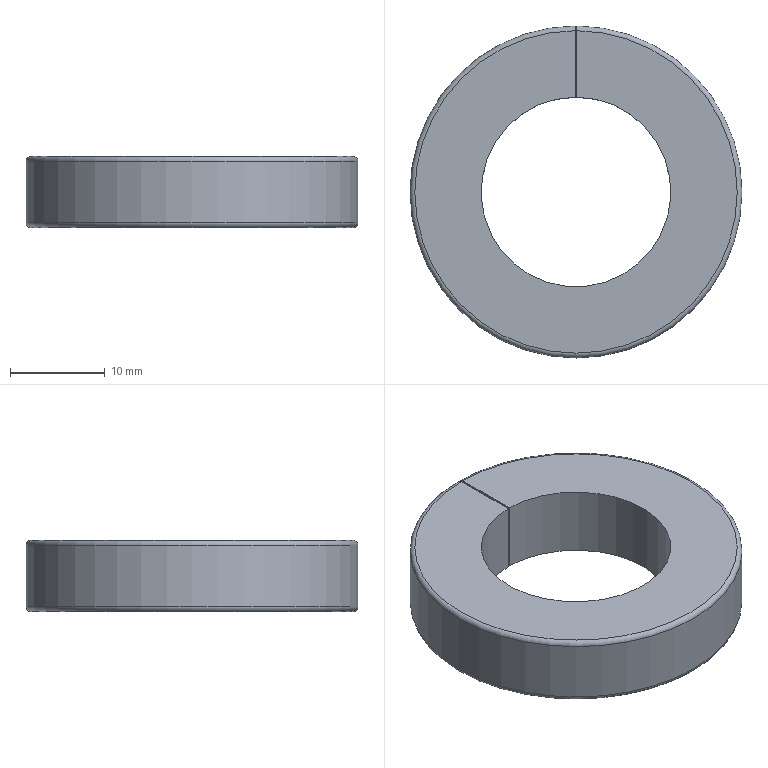Part | NX | features DATUM_CSYS 2, BLEND 1, EXTRUDE 1, SKETCH 1 | 1 solid | 8 faces | box 35 x 35 x 7.5 mm | volume 4837 mm3 | plane 4 | cylinder 2 | torus 2 | commonest cylinder face diameters 20 x1 35 x1
STEP:
#1=CARTESIAN_POINT('',(-0.1,9.999,0.));
#2=VERTEX_POINT('',#1);
#3=CARTESIAN_POINT('',(-0.1,17.,0.));
#4=VERTEX_POINT('',#3);
#5=CARTESIAN_POINT('',(-0.1,9.999,0.));
#6=DIRECTION('',(0.,1.,0.));
#7=VECTOR('',#6,1000.);
#8=LINE('',#5,#7);
#9=EDGE_CURVE('',#2,#4,#8,.T.);
#10=ORIENTED_EDGE('',*,*,#9,.T.);
#11=CARTESIAN_POINT('',(-0.1,17.5,0.5));
#12=VERTEX_POINT('',#11);
#13=CARTESIAN_POINT('',(-0.1,17.,0.));
#14=CARTESIAN_POINT('',(-0.1,17.264,0.));
#15=CARTESIAN_POINT('',(-0.1,17.5,0.2359));
#16=CARTESIAN_POINT('',(-0.1,17.5,0.5));
#17=B_SPLINE_CURVE_WITH_KNOTS('',3,(#13,#14,#15,#16),.UNSPECIFIED.,.F.,.F.,(4,4),(0.,0.0007811),.UNSPECIFIED.);
#18=EDGE_CURVE('',#4,#12,#17,.T.);
#19=ORIENTED_EDGE('',*,*,#18,.T.);
#20=CARTESIAN_POINT('',(-0.1,17.5,7.));
#21=VERTEX_POINT('',#20);
#22=CARTESIAN_POINT('',(-0.1,17.5,7.5));
#23=DIRECTION('',(0.,0.,-1.));
#24=VECTOR('',#23,1000.);
#25=LINE('',#22,#24);
#26=EDGE_CURVE('',#21,#12,#25,.T.);
#27=ORIENTED_EDGE('',*,*,#26,.F.);
#28=CARTESIAN_POINT('',(-0.1,17.,7.5));
#29=VERTEX_POINT('',#28);
#30=CARTESIAN_POINT('',(-0.1,17.5,7.));
#31=CARTESIAN_POINT('',(-0.1,17.5,7.264));
#32=CARTESIAN_POINT('',(-0.1,17.264,7.5));
#33=CARTESIAN_POINT('',(-0.1,17.,7.5));
#34=B_SPLINE_CURVE_WITH_KNOTS('',3,(#30,#31,#32,#33),.UNSPECIFIED.,.F.,.F.,(4,4),(0.,0.0007811),.UNSPECIFIED.);
#35=EDGE_CURVE('',#21,#29,#34,.T.);
#36=ORIENTED_EDGE('',*,*,#35,.T.);
#37=CARTESIAN_POINT('',(-0.1,9.999,7.5));
#38=VERTEX_POINT('',#37);
#39=CARTESIAN_POINT('',(-0.1,9.999,7.5));
#40=DIRECTION('',(0.,1.,0.));
#41=VECTOR('',#40,1000.);
#42=LINE('',#39,#41);
#43=EDGE_CURVE('',#38,#29,#42,.T.);
#44=ORIENTED_EDGE('',*,*,#43,.F.);
#45=CARTESIAN_POINT('',(-0.1,9.999,7.5));
#46=DIRECTION('',(0.,0.,-1.));
#47=VECTOR('',#46,1000.);
#48=LINE('',#45,#47);
#49=EDGE_CURVE('',#38,#2,#48,.T.);
#50=ORIENTED_EDGE('',*,*,#49,.T.);
#51=EDGE_LOOP('',(#10,#19,#27,#36,#44,#50));
#52=FACE_BOUND('',#51,.T.);
#53=CARTESIAN_POINT('',(-0.1,9.999,7.5));
#54=DIRECTION('',(-1.,0.,0.));
#55=DIRECTION('',(0.,0.,1.));
#56=AXIS2_PLACEMENT_3D('',#53,#54,#55);
#57=PLANE('',#56);
#58=ADVANCED_FACE('',(#52),#57,.F.);
#59=ORIENTED_EDGE('',*,*,#26,.T.);
#60=CARTESIAN_POINT('',(0.1,17.5,0.5));
#61=VERTEX_POINT('',#60);
#62=CARTESIAN_POINT('',(0.,0.,0.5));
#63=DIRECTION('',(0.,0.,1.));
#64=DIRECTION('',(1.,0.,0.));
#65=AXIS2_PLACEMENT_3D('',#62,#63,#64);
#66=CIRCLE('',#65,17.5);
#67=EDGE_CURVE('',#12,#61,#66,.T.);
#68=ORIENTED_EDGE('',*,*,#67,.T.);
#69=CARTESIAN_POINT('',(0.1,17.5,7.));
#70=VERTEX_POINT('',#69);
#71=CARTESIAN_POINT('',(0.1,17.5,7.5));
#72=DIRECTION('',(0.,0.,-1.));
#73=VECTOR('',#72,1000.);
#74=LINE('',#71,#73);
#75=EDGE_CURVE('',#70,#61,#74,.T.);
#76=ORIENTED_EDGE('',*,*,#75,.F.);
#77=CARTESIAN_POINT('',(0.,0.,7.));
#78=DIRECTION('',(0.,0.,1.));
#79=DIRECTION('',(1.,0.,0.));
#80=AXIS2_PLACEMENT_3D('',#77,#78,#79);
#81=CIRCLE('',#80,17.5);
#82=EDGE_CURVE('',#70,#21,#81,.F.);
#83=ORIENTED_EDGE('',*,*,#82,.T.);
#84=EDGE_LOOP('',(#59,#68,#76,#83));
#85=FACE_BOUND('',#84,.T.);
#86=CARTESIAN_POINT('',(0.,0.,7.5));
#87=DIRECTION('',(0.,0.,-1.));
#88=DIRECTION('',(-1.,0.,0.));
#89=AXIS2_PLACEMENT_3D('',#86,#87,#88);
#90=CYLINDRICAL_SURFACE('',#89,17.5);
#91=ADVANCED_FACE('',(#85),#90,.T.);
#92=ORIENTED_EDGE('',*,*,#75,.T.);
#93=CARTESIAN_POINT('',(0.1,17.,0.));
#94=VERTEX_POINT('',#93);
#95=CARTESIAN_POINT('',(0.1,17.5,0.5));
#96=CARTESIAN_POINT('',(0.1,17.5,0.2359));
#97=CARTESIAN_POINT('',(0.1,17.264,0.));
#98=CARTESIAN_POINT('',(0.1,17.,0.));
#99=B_SPLINE_CURVE_WITH_KNOTS('',3,(#95,#96,#97,#98),.UNSPECIFIED.,.F.,.F.,(4,4),(0.,0.0007811),.UNSPECIFIED.);
#100=EDGE_CURVE('',#61,#94,#99,.T.);
#101=ORIENTED_EDGE('',*,*,#100,.T.);
#102=CARTESIAN_POINT('',(0.1,9.999,0.));
#103=VERTEX_POINT('',#102);
#104=CARTESIAN_POINT('',(0.1,17.5,0.));
#105=DIRECTION('',(0.,-1.,0.));
#106=VECTOR('',#105,1000.);
#107=LINE('',#104,#106);
#108=EDGE_CURVE('',#94,#103,#107,.T.);
#109=ORIENTED_EDGE('',*,*,#108,.T.);
#110=CARTESIAN_POINT('',(0.1,9.999,7.5));
#111=VERTEX_POINT('',#110);
#112=CARTESIAN_POINT('',(0.1,9.999,7.5));
#113=DIRECTION('',(0.,0.,-1.));
#114=VECTOR('',#113,1000.);
#115=LINE('',#112,#114);
#116=EDGE_CURVE('',#111,#103,#115,.T.);
#117=ORIENTED_EDGE('',*,*,#116,.F.);
#118=CARTESIAN_POINT('',(0.1,17.,7.5));
#119=VERTEX_POINT('',#118);
#120=CARTESIAN_POINT('',(0.1,17.5,7.5));
#121=DIRECTION('',(0.,-1.,0.));
#122=VECTOR('',#121,1000.);
#123=LINE('',#120,#122);
#124=EDGE_CURVE('',#119,#111,#123,.T.);
#125=ORIENTED_EDGE('',*,*,#124,.F.);
#126=CARTESIAN_POINT('',(0.1,17.,7.5));
#127=CARTESIAN_POINT('',(0.1,17.264,7.5));
#128=CARTESIAN_POINT('',(0.1,17.5,7.264));
#129=CARTESIAN_POINT('',(0.1,17.5,7.));
#130=B_SPLINE_CURVE_WITH_KNOTS('',3,(#126,#127,#128,#129),.UNSPECIFIED.,.F.,.F.,(4,4),(0.,0.0007811),.UNSPECIFIED.);
#131=EDGE_CURVE('',#119,#70,#130,.T.);
#132=ORIENTED_EDGE('',*,*,#131,.T.);
#133=EDGE_LOOP('',(#92,#101,#109,#117,#125,#132));
#134=FACE_BOUND('',#133,.T.);
#135=CARTESIAN_POINT('',(0.1,17.5,7.5));
#136=DIRECTION('',(1.,0.,0.));
#137=DIRECTION('',(0.,0.,-1.));
#138=AXIS2_PLACEMENT_3D('',#135,#136,#137);
#139=PLANE('',#138);
#140=ADVANCED_FACE('',(#134),#139,.F.);
#141=CARTESIAN_POINT('',(0.,0.,0.));
#142=DIRECTION('',(0.,0.,-1.));
#143=DIRECTION('',(1.,0.,0.));
#144=AXIS2_PLACEMENT_3D('',#141,#142,#143);
#145=CIRCLE('',#144,10.);
#146=EDGE_CURVE('',#103,#2,#145,.T.);
#147=ORIENTED_EDGE('',*,*,#146,.T.);
#148=ORIENTED_EDGE('',*,*,#49,.F.);
#149=CARTESIAN_POINT('',(0.,0.,7.5));
#150=DIRECTION('',(0.,0.,-1.));
#151=DIRECTION('',(1.,0.,0.));
#152=AXIS2_PLACEMENT_3D('',#149,#150,#151);
#153=CIRCLE('',#152,10.);
#154=EDGE_CURVE('',#111,#38,#153,.T.);
#155=ORIENTED_EDGE('',*,*,#154,.F.);
#156=ORIENTED_EDGE('',*,*,#116,.T.);
#157=EDGE_LOOP('',(#147,#148,#155,#156));
#158=FACE_BOUND('',#157,.T.);
#159=CARTESIAN_POINT('',(0.,0.,7.5));
#160=DIRECTION('',(0.,0.,-1.));
#161=DIRECTION('',(-1.,0.,0.));
#162=AXIS2_PLACEMENT_3D('',#159,#160,#161);
#163=CYLINDRICAL_SURFACE('',#162,10.);
#164=ADVANCED_FACE('',(#158),#163,.F.);
#165=ORIENTED_EDGE('',*,*,#43,.T.);
#166=CARTESIAN_POINT('',(0.,0.,7.5));
#167=DIRECTION('',(0.,0.,1.));
#168=DIRECTION('',(1.,0.,0.));
#169=AXIS2_PLACEMENT_3D('',#166,#167,#168);
#170=CIRCLE('',#169,17.);
#171=EDGE_CURVE('',#29,#119,#170,.T.);
#172=ORIENTED_EDGE('',*,*,#171,.T.);
#173=ORIENTED_EDGE('',*,*,#124,.T.);
#174=ORIENTED_EDGE('',*,*,#154,.T.);
#175=EDGE_LOOP('',(#165,#172,#173,#174));
#176=FACE_BOUND('',#175,.T.);
#177=CARTESIAN_POINT('',(0.,0.,7.5));
#178=DIRECTION('',(0.,0.,1.));
#179=DIRECTION('',(1.,0.,0.));
#180=AXIS2_PLACEMENT_3D('',#177,#178,#179);
#181=PLANE('',#180);
#182=ADVANCED_FACE('',(#176),#181,.T.);
#183=ORIENTED_EDGE('',*,*,#108,.F.);
#184=CARTESIAN_POINT('',(0.,0.,0.));
#185=DIRECTION('',(0.,0.,1.));
#186=DIRECTION('',(1.,0.,0.));
#187=AXIS2_PLACEMENT_3D('',#184,#185,#186);
#188=CIRCLE('',#187,17.);
#189=EDGE_CURVE('',#94,#4,#188,.F.);
#190=ORIENTED_EDGE('',*,*,#189,.T.);
#191=ORIENTED_EDGE('',*,*,#9,.F.);
#192=ORIENTED_EDGE('',*,*,#146,.F.);
#193=EDGE_LOOP('',(#183,#190,#191,#192));
#194=FACE_BOUND('',#193,.T.);
#195=CARTESIAN_POINT('',(0.,0.,0.));
#196=DIRECTION('',(0.,0.,1.));
#197=DIRECTION('',(1.,0.,0.));
#198=AXIS2_PLACEMENT_3D('',#195,#196,#197);
#199=PLANE('',#198);
#200=ADVANCED_FACE('',(#194),#199,.F.);
#201=ORIENTED_EDGE('',*,*,#18,.F.);
#202=ORIENTED_EDGE('',*,*,#189,.F.);
#203=ORIENTED_EDGE('',*,*,#100,.F.);
#204=ORIENTED_EDGE('',*,*,#67,.F.);
#205=EDGE_LOOP('',(#201,#202,#203,#204));
#206=FACE_BOUND('',#205,.T.);
#207=CARTESIAN_POINT('',(0.,0.,0.5));
#208=DIRECTION('',(0.,0.,1.));
#209=DIRECTION('',(1.,0.,0.));
#210=AXIS2_PLACEMENT_3D('',#207,#208,#209);
#211=TOROIDAL_SURFACE('',#210,17.,0.5);
#212=ADVANCED_FACE('',(#206),#211,.T.);
#213=ORIENTED_EDGE('',*,*,#35,.F.);
#214=ORIENTED_EDGE('',*,*,#82,.F.);
#215=ORIENTED_EDGE('',*,*,#131,.F.);
#216=ORIENTED_EDGE('',*,*,#171,.F.);
#217=EDGE_LOOP('',(#213,#214,#215,#216));
#218=FACE_BOUND('',#217,.T.);
#219=CARTESIAN_POINT('',(0.,0.,7.));
#220=DIRECTION('',(0.,0.,1.));
#221=DIRECTION('',(1.,0.,0.));
#222=AXIS2_PLACEMENT_3D('',#219,#220,#221);
#223=TOROIDAL_SURFACE('',#222,17.,0.5);
#224=ADVANCED_FACE('',(#218),#223,.T.);
#225=CLOSED_SHELL('',(#58,#91,#140,#164,#182,#200,#212,#224));
#226=MANIFOLD_SOLID_BREP('',#225);
#227=(LENGTH_UNIT()NAMED_UNIT(*)SI_UNIT(.MILLI.,.METRE.));
#228=UNCERTAINTY_MEASURE_WITH_UNIT(LENGTH_MEASURE(0.0508),#227,'','');
#229=(NAMED_UNIT(*)PLANE_ANGLE_UNIT()SI_UNIT($,.RADIAN.));
#230=(NAMED_UNIT(*)SI_UNIT($,.STERADIAN.)SOLID_ANGLE_UNIT());
#231=(GEOMETRIC_REPRESENTATION_CONTEXT(3)GLOBAL_UNCERTAINTY_ASSIGNED_CONTEXT((#228))GLOBAL_UNIT_ASSIGNED_CONTEXT((#227,#229,#230))REPRESENTATION_CONTEXT('',''));
#232=ADVANCED_BREP_SHAPE_REPRESENTATION('',(#226),#231);